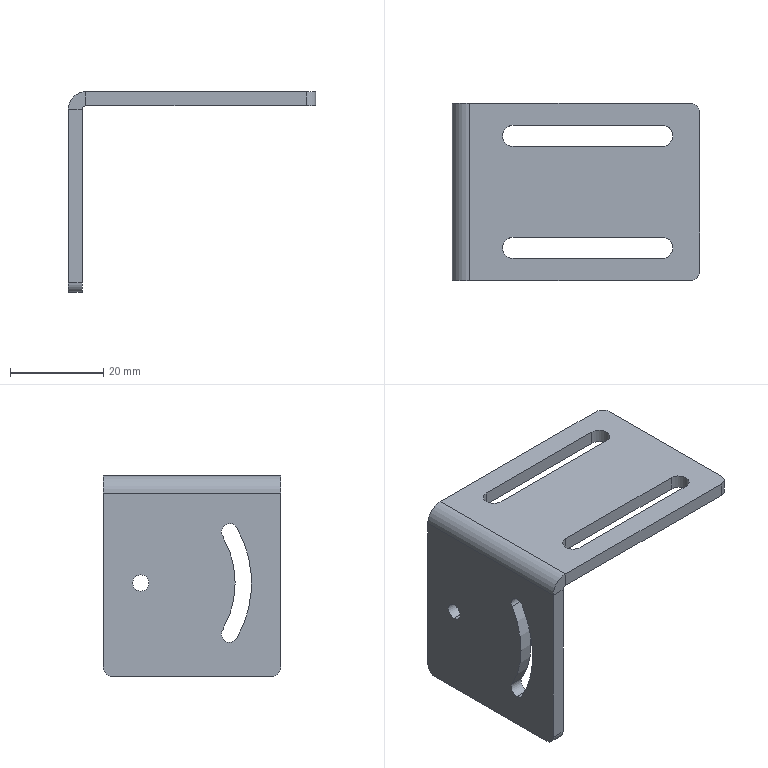Part | STEP file | ND25021-01-JDKM-05-BJ | 1 solid | 35 faces | box 53 x 38 x 43 mm | volume 9223 mm3 | cylinder 19 | plane 16 | commonest cylinder face diameters 4.5 x6 3.5 x5 4 x4 1.473 x1 7.473 x1 40.5 x1